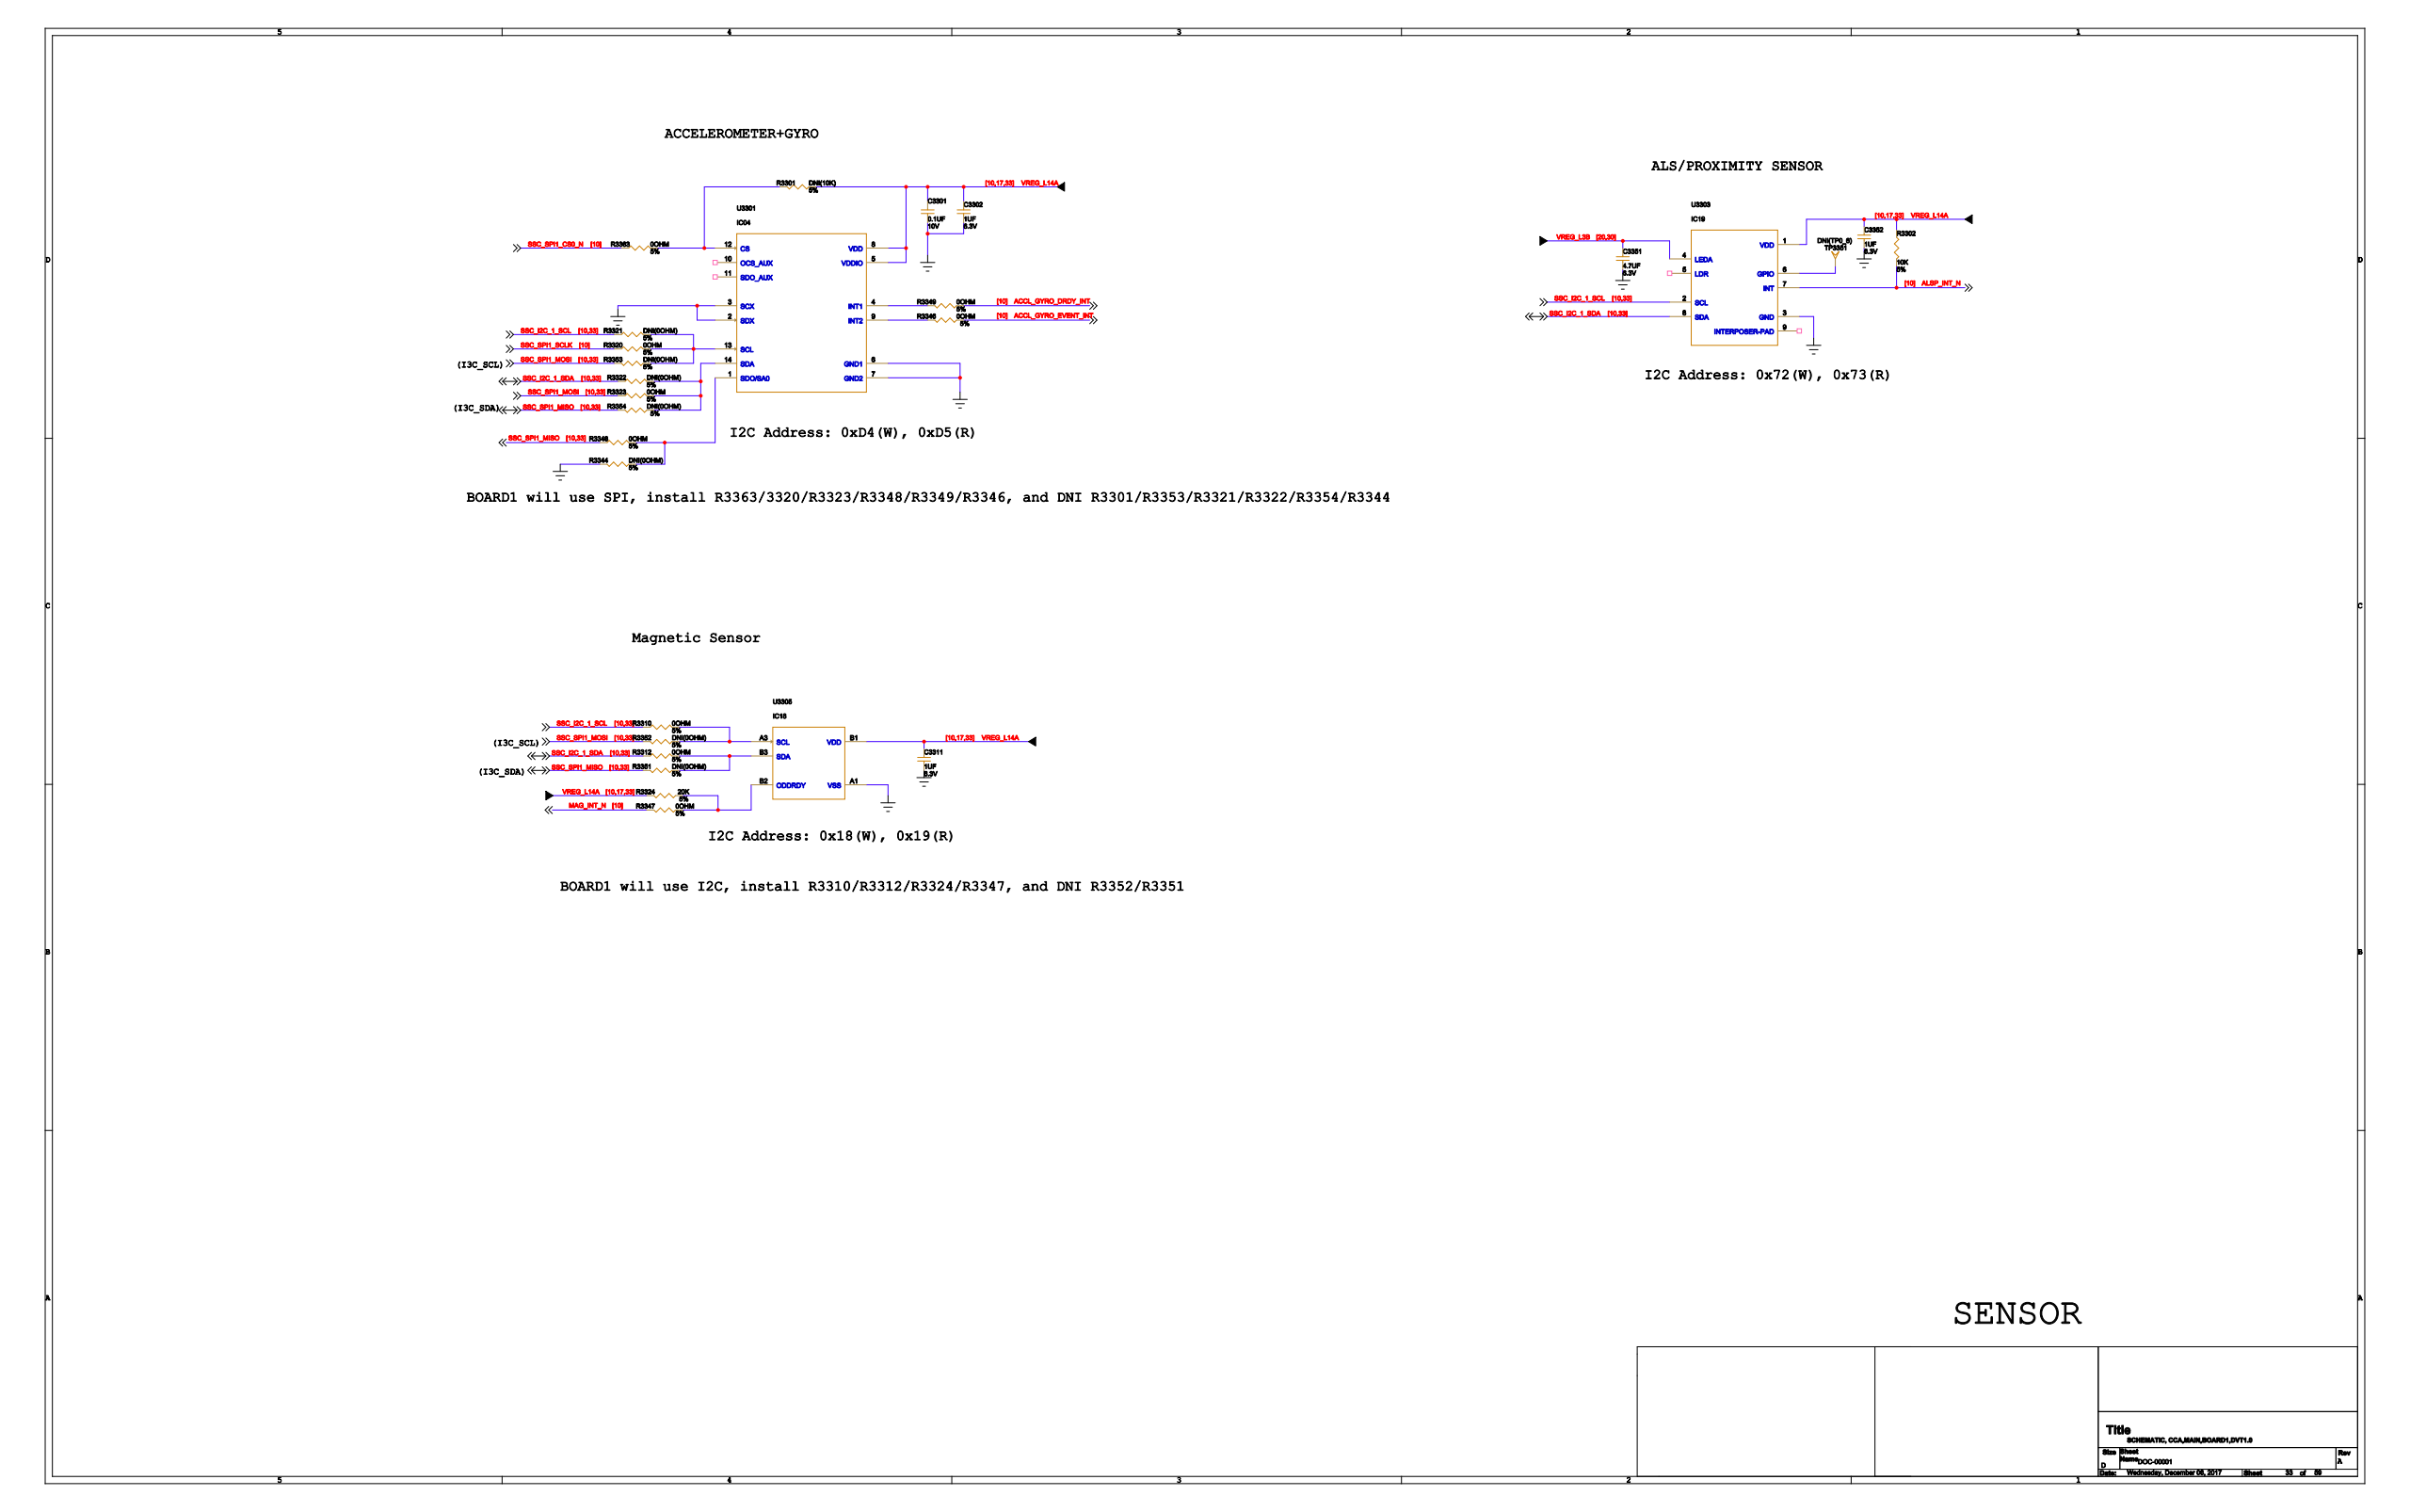Circuit board | KiCad | 1657 parts | 1365 nets | one sheet of the schematic
Parts on this sheet (reference | value | footprint):
C3301
C3302
C3311
C3351
C3352
R3301
R3302
R3310
R3312
R3320
R3321
R3322
R3323
R3324
R3344
R3346
R3347
R3348
R3349
R3351
R3352
R3353
R3354
R3363
TP3351
U3301
U3303
U3305
Nets of these parts (net: part-pin ...):
GND: C3301-2 C3302-2 C3311-2 C3351-2 C3352-2 R3344-1 U3301-2 U3301-3 U3301-6 U3301-7 U3303-3 U3305-A1
N22156852: R3344-2 R3348-2 U3301-1
N23449782: R3310-2 R3352-1 U3305-A3
VREG_L14A: C3301-1 C3302-1 C3311-1 C3352-1 R3301-2 R3302-2 R3324-1 U3301-5 U3301-8 U3303-1 U3305-B1
N22154616: R3324-2 R3347-2 U3305-B2
N18829978: R3312-2 R3351-1 U3305-B3
N22156524: R3320-2 R3321-1 R3353-1 U3301-13
SSC_SPI1_MOSI: R3323-1 R3352-2 R3353-2
N22155346: R3349-1 U3301-4
_GYRO_DRDY_INT: R3349-2
SSC_I2C_1_SDA: R3312-1 R3322-2 U3303-8
N22156518: R3322-1 R3323-2 R3354-1 U3301-14
SSC_SPI1_MISO: R3348-1 R3351-2 R3354-2
N42181376: TP3351-1 U3303-6
N22156996: R3301-1 R3363-2 U3301-12
N22155344: R3346-1 U3301-9
GYRO_EVENT_INT: R3346-2
SSC_SPI1_SCLK: R3320-1
SSC_I2C_1_SCL: R3310-1 R3321-2 U3303-2
SSC_SPI1_CS0_N: R3363-1
MAG_INT_N: R3347-1
ALSP_INT_N: R3302-1 U3303-7
VREG_L3B: C3351-1 U3303-4
NET_1252: U3303-5
NET_1253: U3303-9
NET_351: U3301-10
NET_352: U3301-11